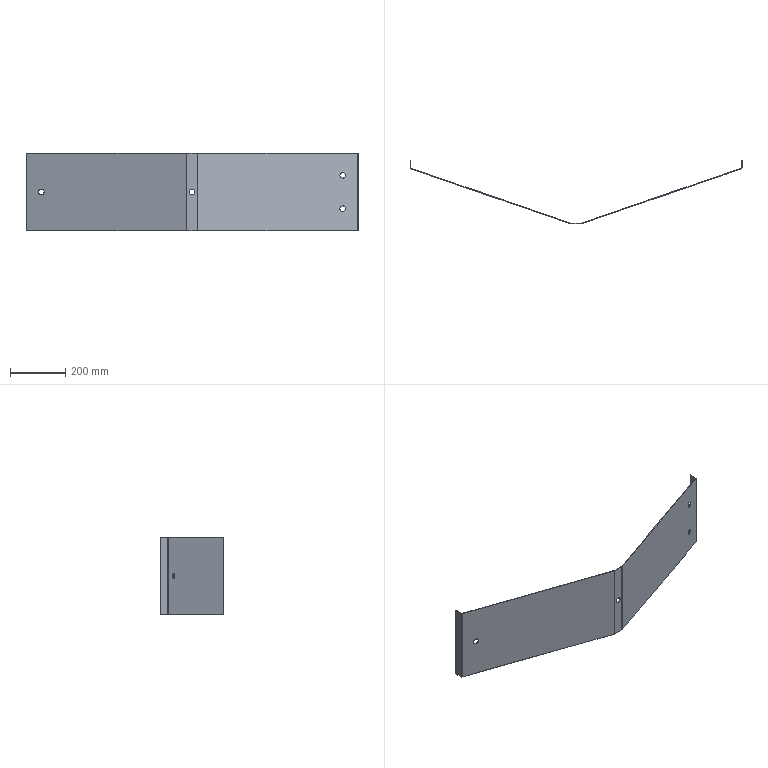Part | SolidWorks | features ICE 4, FlatPattern 1, SMBaseFlange 1, SheetMetal 1 | 1 solid | 46 faces | box 1200 x 230 x 280 mm | volume 738116 mm3 | plane 30 | cylinder 16 | commonest cylinder face diameters 20 x8 2 x4 6 x4
STEP:
#1=CARTESIAN_POINT('',(55.332,-16.965,130.));
#2=VERTEX_POINT('',#1);
#3=CARTESIAN_POINT('',(55.332,-16.965,150.));
#4=VERTEX_POINT('',#3);
#5=CARTESIAN_POINT('',(55.332,-16.965,130.));
#6=CARTESIAN_POINT('',(35.332,-10.068,130.));
#7=CARTESIAN_POINT('',(35.332,-10.068,150.));
#8=CARTESIAN_POINT('',(55.332,-16.965,150.));
#9=(BOUNDED_CURVE()B_SPLINE_CURVE(3,(#5,#6,#7,#8),.UNSPECIFIED.,.F.,.T.)B_SPLINE_CURVE_WITH_KNOTS((4,4),(1.571,4.712),.UNSPECIFIED.)CURVE()GEOMETRIC_REPRESENTATION_ITEM()RATIONAL_B_SPLINE_CURVE((1.,0.3333,0.3333,1.))REPRESENTATION_ITEM(''));
#10=EDGE_CURVE('',#2,#4,#9,.T.);
#11=ORIENTED_EDGE('',*,*,#10,.T.);
#12=CARTESIAN_POINT('',(55.332,-19.08,150.));
#13=VERTEX_POINT('',#12);
#14=CARTESIAN_POINT('',(55.332,30.,150.));
#15=DIRECTION('',(0.,-1.,0.));
#16=VECTOR('',#15,1000.);
#17=LINE('',#14,#16);
#18=EDGE_CURVE('',#4,#13,#17,.T.);
#19=ORIENTED_EDGE('',*,*,#18,.T.);
#20=CARTESIAN_POINT('',(55.332,-19.08,130.));
#21=VERTEX_POINT('',#20);
#22=CARTESIAN_POINT('',(55.332,-19.08,130.));
#23=CARTESIAN_POINT('',(35.332,-12.184,130.));
#24=CARTESIAN_POINT('',(35.332,-12.184,150.));
#25=CARTESIAN_POINT('',(55.332,-19.08,150.));
#26=(BOUNDED_CURVE()B_SPLINE_CURVE(3,(#22,#23,#24,#25),.UNSPECIFIED.,.F.,.F.)B_SPLINE_CURVE_WITH_KNOTS((4,4),(1.571,4.712),.UNSPECIFIED.)CURVE()GEOMETRIC_REPRESENTATION_ITEM()RATIONAL_B_SPLINE_CURVE((1.,0.3333,0.3333,1.))REPRESENTATION_ITEM(''));
#27=EDGE_CURVE('',#21,#13,#26,.T.);
#28=ORIENTED_EDGE('',*,*,#27,.F.);
#29=CARTESIAN_POINT('',(55.332,30.,130.));
#30=DIRECTION('',(0.,-1.,0.));
#31=VECTOR('',#30,1000.);
#32=LINE('',#29,#31);
#33=EDGE_CURVE('',#2,#21,#32,.T.);
#34=ORIENTED_EDGE('',*,*,#33,.F.);
#35=EDGE_LOOP('',(#11,#19,#28,#34));
#36=FACE_OUTER_BOUND('',#35,.T.);
#37=CARTESIAN_POINT('',(55.332,30.,140.));
#38=DIRECTION('',(0.,-1.,0.));
#39=DIRECTION('',(0.,0.,-1.));
#40=AXIS2_PLACEMENT_3D('',#37,#38,#39);
#41=CYLINDRICAL_SURFACE('',#40,10.);
#42=ADVANCED_FACE('',(#36),#41,.F.);
#43=CARTESIAN_POINT('',(1144.668,-16.965,190.));
#44=VERTEX_POINT('',#43);
#45=CARTESIAN_POINT('',(1144.668,-16.965,210.));
#46=VERTEX_POINT('',#45);
#47=CARTESIAN_POINT('',(1144.668,-16.965,190.));
#48=CARTESIAN_POINT('',(1124.668,-23.861,190.));
#49=CARTESIAN_POINT('',(1124.668,-23.861,210.));
#50=CARTESIAN_POINT('',(1144.668,-16.965,210.));
#51=(BOUNDED_CURVE()B_SPLINE_CURVE(3,(#47,#48,#49,#50),.UNSPECIFIED.,.F.,.T.)B_SPLINE_CURVE_WITH_KNOTS((4,4),(4.712,7.854),.UNSPECIFIED.)CURVE()GEOMETRIC_REPRESENTATION_ITEM()RATIONAL_B_SPLINE_CURVE((1.,0.3333,0.3333,1.))REPRESENTATION_ITEM(''));
#52=EDGE_CURVE('',#44,#46,#51,.T.);
#53=ORIENTED_EDGE('',*,*,#52,.T.);
#54=CARTESIAN_POINT('',(1144.668,-19.08,210.));
#55=VERTEX_POINT('',#54);
#56=CARTESIAN_POINT('',(1144.668,30.,210.));
#57=DIRECTION('',(0.,-1.,0.));
#58=VECTOR('',#57,1000.);
#59=LINE('',#56,#58);
#60=EDGE_CURVE('',#46,#55,#59,.T.);
#61=ORIENTED_EDGE('',*,*,#60,.T.);
#62=CARTESIAN_POINT('',(1144.668,-19.08,190.));
#63=VERTEX_POINT('',#62);
#64=CARTESIAN_POINT('',(1144.668,-19.08,190.));
#65=CARTESIAN_POINT('',(1124.668,-25.977,190.));
#66=CARTESIAN_POINT('',(1124.668,-25.977,210.));
#67=CARTESIAN_POINT('',(1144.668,-19.08,210.));
#68=(BOUNDED_CURVE()B_SPLINE_CURVE(3,(#64,#65,#66,#67),.UNSPECIFIED.,.F.,.F.)B_SPLINE_CURVE_WITH_KNOTS((4,4),(4.712,7.854),.UNSPECIFIED.)CURVE()GEOMETRIC_REPRESENTATION_ITEM()RATIONAL_B_SPLINE_CURVE((1.,0.3333,0.3333,1.))REPRESENTATION_ITEM(''));
#69=EDGE_CURVE('',#63,#55,#68,.T.);
#70=ORIENTED_EDGE('',*,*,#69,.F.);
#71=CARTESIAN_POINT('',(1144.668,30.,190.));
#72=DIRECTION('',(0.,-1.,0.));
#73=VECTOR('',#72,1000.);
#74=LINE('',#71,#73);
#75=EDGE_CURVE('',#44,#63,#74,.T.);
#76=ORIENTED_EDGE('',*,*,#75,.F.);
#77=EDGE_LOOP('',(#53,#61,#70,#76));
#78=FACE_OUTER_BOUND('',#77,.T.);
#79=CARTESIAN_POINT('',(1144.668,30.,200.));
#80=DIRECTION('',(0.,-1.,0.));
#81=DIRECTION('',(0.,0.,-1.));
#82=AXIS2_PLACEMENT_3D('',#79,#80,#81);
#83=CYLINDRICAL_SURFACE('',#82,10.);
#84=ADVANCED_FACE('',(#78),#83,.F.);
#85=CARTESIAN_POINT('',(1144.668,-16.965,70.));
#86=VERTEX_POINT('',#85);
#87=CARTESIAN_POINT('',(1144.668,-16.965,90.));
#88=VERTEX_POINT('',#87);
#89=CARTESIAN_POINT('',(1144.668,-16.965,70.));
#90=CARTESIAN_POINT('',(1124.668,-23.861,70.));
#91=CARTESIAN_POINT('',(1124.668,-23.861,90.));
#92=CARTESIAN_POINT('',(1144.668,-16.965,90.));
#93=(BOUNDED_CURVE()B_SPLINE_CURVE(3,(#89,#90,#91,#92),.UNSPECIFIED.,.F.,.T.)B_SPLINE_CURVE_WITH_KNOTS((4,4),(4.712,7.854),.UNSPECIFIED.)CURVE()GEOMETRIC_REPRESENTATION_ITEM()RATIONAL_B_SPLINE_CURVE((1.,0.3333,0.3333,1.))REPRESENTATION_ITEM(''));
#94=EDGE_CURVE('',#86,#88,#93,.T.);
#95=ORIENTED_EDGE('',*,*,#94,.T.);
#96=CARTESIAN_POINT('',(1144.668,-19.08,90.));
#97=VERTEX_POINT('',#96);
#98=CARTESIAN_POINT('',(1144.668,30.,90.));
#99=DIRECTION('',(0.,-1.,0.));
#100=VECTOR('',#99,1000.);
#101=LINE('',#98,#100);
#102=EDGE_CURVE('',#88,#97,#101,.T.);
#103=ORIENTED_EDGE('',*,*,#102,.T.);
#104=CARTESIAN_POINT('',(1144.668,-19.08,70.));
#105=VERTEX_POINT('',#104);
#106=CARTESIAN_POINT('',(1144.668,-19.08,70.));
#107=CARTESIAN_POINT('',(1124.668,-25.977,70.));
#108=CARTESIAN_POINT('',(1124.668,-25.977,90.));
#109=CARTESIAN_POINT('',(1144.668,-19.08,90.));
#110=(BOUNDED_CURVE()B_SPLINE_CURVE(3,(#106,#107,#108,#109),.UNSPECIFIED.,.F.,.F.)B_SPLINE_CURVE_WITH_KNOTS((4,4),(4.712,7.854),.UNSPECIFIED.)CURVE()GEOMETRIC_REPRESENTATION_ITEM()RATIONAL_B_SPLINE_CURVE((1.,0.3333,0.3333,1.))REPRESENTATION_ITEM(''));
#111=EDGE_CURVE('',#105,#97,#110,.T.);
#112=ORIENTED_EDGE('',*,*,#111,.F.);
#113=CARTESIAN_POINT('',(1144.668,30.,70.));
#114=DIRECTION('',(0.,-1.,0.));
#115=VECTOR('',#114,1000.);
#116=LINE('',#113,#115);
#117=EDGE_CURVE('',#86,#105,#116,.T.);
#118=ORIENTED_EDGE('',*,*,#117,.F.);
#119=EDGE_LOOP('',(#95,#103,#112,#118));
#120=FACE_OUTER_BOUND('',#119,.T.);
#121=CARTESIAN_POINT('',(1144.668,30.,80.));
#122=DIRECTION('',(0.,-1.,0.));
#123=DIRECTION('',(0.,0.,-1.));
#124=AXIS2_PLACEMENT_3D('',#121,#122,#123);
#125=CYLINDRICAL_SURFACE('',#124,10.);
#126=ADVANCED_FACE('',(#120),#125,.F.);
#127=CARTESIAN_POINT('',(600.,-200.,130.));
#128=VERTEX_POINT('',#127);
#129=CARTESIAN_POINT('',(600.,-200.,150.));
#130=VERTEX_POINT('',#129);
#131=CARTESIAN_POINT('',(600.,-200.,140.));
#132=DIRECTION('',(0.,1.,0.));
#133=DIRECTION('',(0.,0.,1.));
#134=AXIS2_PLACEMENT_3D('',#131,#132,#133);
#135=CIRCLE('',#134,10.);
#136=EDGE_CURVE('',#128,#130,#135,.T.);
#137=ORIENTED_EDGE('',*,*,#136,.F.);
#138=CARTESIAN_POINT('',(600.,-198.,130.));
#139=VERTEX_POINT('',#138);
#140=CARTESIAN_POINT('',(600.,-208.,130.));
#141=DIRECTION('',(0.,1.,0.));
#142=VECTOR('',#141,1000.);
#143=LINE('',#140,#142);
#144=EDGE_CURVE('',#128,#139,#143,.T.);
#145=ORIENTED_EDGE('',*,*,#144,.T.);
#146=CARTESIAN_POINT('',(600.,-198.,150.));
#147=VERTEX_POINT('',#146);
#148=CARTESIAN_POINT('',(600.,-198.,140.));
#149=DIRECTION('',(0.,1.,0.));
#150=DIRECTION('',(0.,0.,1.));
#151=AXIS2_PLACEMENT_3D('',#148,#149,#150);
#152=CIRCLE('',#151,10.);
#153=EDGE_CURVE('',#139,#147,#152,.T.);
#154=ORIENTED_EDGE('',*,*,#153,.T.);
#155=CARTESIAN_POINT('',(600.,-208.,150.));
#156=DIRECTION('',(0.,1.,0.));
#157=VECTOR('',#156,1000.);
#158=LINE('',#155,#157);
#159=EDGE_CURVE('',#130,#147,#158,.T.);
#160=ORIENTED_EDGE('',*,*,#159,.F.);
#161=EDGE_LOOP('',(#137,#145,#154,#160));
#162=FACE_OUTER_BOUND('',#161,.T.);
#163=CARTESIAN_POINT('',(600.,-208.,140.));
#164=DIRECTION('',(0.,1.,0.));
#165=DIRECTION('',(0.,0.,1.));
#166=AXIS2_PLACEMENT_3D('',#163,#164,#165);
#167=CYLINDRICAL_SURFACE('',#166,10.);
#168=ADVANCED_FACE('',(#162),#167,.F.);
#169=CARTESIAN_POINT('',(0.,2.139,280.));
#170=VERTEX_POINT('',#169);
#171=CARTESIAN_POINT('',(2.,2.139,280.));
#172=VERTEX_POINT('',#171);
#173=CARTESIAN_POINT('',(0.,2.139,280.));
#174=DIRECTION('',(1.,0.,0.));
#175=VECTOR('',#174,1000.);
#176=LINE('',#173,#175);
#177=EDGE_CURVE('',#170,#172,#176,.T.);
#178=ORIENTED_EDGE('',*,*,#177,.F.);
#179=CARTESIAN_POINT('',(2.022,-0.6973,280.));
#180=VERTEX_POINT('',#179);
#181=CARTESIAN_POINT('',(3.,2.139,280.));
#182=DIRECTION('',(0.,0.,1.));
#183=DIRECTION('',(-1.,0.,0.));
#184=AXIS2_PLACEMENT_3D('',#181,#182,#183);
#185=CIRCLE('',#184,3.);
#186=EDGE_CURVE('',#170,#180,#185,.T.);
#187=ORIENTED_EDGE('',*,*,#186,.T.);
#188=CARTESIAN_POINT('',(2.674,1.193,280.));
#189=VERTEX_POINT('',#188);
#190=CARTESIAN_POINT('',(2.674,1.193,280.));
#191=DIRECTION('',(-0.326,-0.9454,0.));
#192=VECTOR('',#191,1000.);
#193=LINE('',#190,#192);
#194=EDGE_CURVE('',#189,#180,#193,.T.);
#195=ORIENTED_EDGE('',*,*,#194,.F.);
#196=CARTESIAN_POINT('',(3.,2.139,280.));
#197=DIRECTION('',(0.,0.,1.));
#198=DIRECTION('',(1.,0.,0.));
#199=AXIS2_PLACEMENT_3D('',#196,#197,#198);
#200=CIRCLE('',#199,1.);
#201=EDGE_CURVE('',#172,#189,#200,.T.);
#202=ORIENTED_EDGE('',*,*,#201,.F.);
#203=EDGE_LOOP('',(#178,#187,#195,#202));
#204=FACE_OUTER_BOUND('',#203,.T.);
#205=CARTESIAN_POINT('',(0.,2.139,280.));
#206=DIRECTION('',(0.,0.,1.));
#207=DIRECTION('',(1.,0.,0.));
#208=AXIS2_PLACEMENT_3D('',#205,#206,#207);
#209=PLANE('',#208);
#210=ADVANCED_FACE('',(#204),#209,.T.);
#211=CARTESIAN_POINT('',(0.,30.,280.));
#212=VERTEX_POINT('',#211);
#213=CARTESIAN_POINT('',(0.,0.,280.));
#214=DIRECTION('',(0.,-1.,0.));
#215=VECTOR('',#214,1000.);
#216=LINE('',#213,#215);
#217=EDGE_CURVE('',#212,#170,#216,.T.);
#218=ORIENTED_EDGE('',*,*,#217,.T.);
#219=ORIENTED_EDGE('',*,*,#177,.T.);
#220=CARTESIAN_POINT('',(2.,30.,280.));
#221=VERTEX_POINT('',#220);
#222=CARTESIAN_POINT('',(2.,0.,280.));
#223=DIRECTION('',(0.,-1.,0.));
#224=VECTOR('',#223,1000.);
#225=LINE('',#222,#224);
#226=EDGE_CURVE('',#221,#172,#225,.T.);
#227=ORIENTED_EDGE('',*,*,#226,.F.);
#228=CARTESIAN_POINT('',(0.,30.,280.));
#229=DIRECTION('',(1.,0.,0.));
#230=VECTOR('',#229,1000.);
#231=LINE('',#228,#230);
#232=EDGE_CURVE('',#212,#221,#231,.T.);
#233=ORIENTED_EDGE('',*,*,#232,.F.);
#234=EDGE_LOOP('',(#218,#219,#227,#233));
#235=FACE_OUTER_BOUND('',#234,.T.);
#236=CARTESIAN_POINT('',(2.674,1.193,280.));
#237=DIRECTION('',(0.,0.,1.));
#238=DIRECTION('',(1.,0.,0.));
#239=AXIS2_PLACEMENT_3D('',#236,#237,#238);
#240=PLANE('',#239);
#241=ADVANCED_FACE('',(#235),#240,.T.);
#242=CARTESIAN_POINT('',(2.022,-0.6973,0.));
#243=VERTEX_POINT('',#242);
#244=CARTESIAN_POINT('',(2.674,1.193,0.));
#245=VERTEX_POINT('',#244);
#246=CARTESIAN_POINT('',(2.022,-0.6973,0.));
#247=DIRECTION('',(0.326,0.9454,0.));
#248=VECTOR('',#247,1000.);
#249=LINE('',#246,#248);
#250=EDGE_CURVE('',#243,#245,#249,.T.);
#251=ORIENTED_EDGE('',*,*,#250,.F.);
#252=CARTESIAN_POINT('',(0.,2.139,0.));
#253=VERTEX_POINT('',#252);
#254=CARTESIAN_POINT('',(3.,2.139,0.));
#255=DIRECTION('',(0.,0.,1.));
#256=DIRECTION('',(-1.,0.,0.));
#257=AXIS2_PLACEMENT_3D('',#254,#255,#256);
#258=CIRCLE('',#257,3.);
#259=EDGE_CURVE('',#253,#243,#258,.T.);
#260=ORIENTED_EDGE('',*,*,#259,.F.);
#261=CARTESIAN_POINT('',(2.,2.139,0.));
#262=VERTEX_POINT('',#261);
#263=CARTESIAN_POINT('',(2.,2.139,0.));
#264=DIRECTION('',(-1.,0.,0.));
#265=VECTOR('',#264,1000.);
#266=LINE('',#263,#265);
#267=EDGE_CURVE('',#262,#253,#266,.T.);
#268=ORIENTED_EDGE('',*,*,#267,.F.);
#269=CARTESIAN_POINT('',(3.,2.139,0.));
#270=DIRECTION('',(0.,0.,1.));
#271=DIRECTION('',(1.,0.,0.));
#272=AXIS2_PLACEMENT_3D('',#269,#270,#271);
#273=CIRCLE('',#272,1.);
#274=EDGE_CURVE('',#262,#245,#273,.T.);
#275=ORIENTED_EDGE('',*,*,#274,.T.);
#276=EDGE_LOOP('',(#251,#260,#268,#275));
#277=FACE_OUTER_BOUND('',#276,.T.);
#278=CARTESIAN_POINT('',(2.022,-0.6973,0.));
#279=DIRECTION('',(0.,0.,-1.));
#280=DIRECTION('',(-1.,0.,0.));
#281=AXIS2_PLACEMENT_3D('',#278,#279,#280);
#282=PLANE('',#281);
#283=ADVANCED_FACE('',(#277),#282,.T.);
#284=CARTESIAN_POINT('',(579.525,-199.836,0.));
#285=VERTEX_POINT('',#284);
#286=CARTESIAN_POINT('',(0.,0.,0.));
#287=DIRECTION('',(0.9454,-0.326,0.));
#288=VECTOR('',#287,1000.);
#289=LINE('',#286,#288);
#290=EDGE_CURVE('',#243,#285,#289,.T.);
#291=ORIENTED_EDGE('',*,*,#290,.F.);
#292=ORIENTED_EDGE('',*,*,#250,.T.);
#293=CARTESIAN_POINT('',(580.177,-197.945,0.));
#294=VERTEX_POINT('',#293);
#295=CARTESIAN_POINT('',(0.652,1.891,0.));
#296=DIRECTION('',(0.9454,-0.326,0.));
#297=VECTOR('',#296,1000.);
#298=LINE('',#295,#297);
#299=EDGE_CURVE('',#245,#294,#298,.T.);
#300=ORIENTED_EDGE('',*,*,#299,.T.);
#301=CARTESIAN_POINT('',(580.177,-197.945,0.));
#302=DIRECTION('',(-0.326,-0.9454,0.));
#303=VECTOR('',#302,1000.);
#304=LINE('',#301,#303);
#305=EDGE_CURVE('',#294,#285,#304,.T.);
#306=ORIENTED_EDGE('',*,*,#305,.T.);
#307=EDGE_LOOP('',(#291,#292,#300,#306));
#308=FACE_OUTER_BOUND('',#307,.T.);
#309=CARTESIAN_POINT('',(2.,2.139,0.));
#310=DIRECTION('',(0.,0.,-1.));
#311=DIRECTION('',(-1.,0.,0.));
#312=AXIS2_PLACEMENT_3D('',#309,#310,#311);
#313=PLANE('',#312);
#314=ADVANCED_FACE('',(#308),#313,.T.);
#315=CARTESIAN_POINT('',(579.525,-199.836,280.));
#316=VERTEX_POINT('',#315);
#317=CARTESIAN_POINT('',(580.177,-197.945,280.));
#318=VERTEX_POINT('',#317);
#319=CARTESIAN_POINT('',(579.525,-199.836,280.));
#320=DIRECTION('',(0.326,0.9454,0.));
#321=VECTOR('',#320,1000.);
#322=LINE('',#319,#321);
#323=EDGE_CURVE('',#316,#318,#322,.T.);
#324=ORIENTED_EDGE('',*,*,#323,.F.);
#325=CARTESIAN_POINT('',(580.503,-200.,280.));
#326=VERTEX_POINT('',#325);
#327=CARTESIAN_POINT('',(580.503,-197.,280.));
#328=DIRECTION('',(0.,0.,1.));
#329=DIRECTION('',(-1.,0.,0.));
#330=AXIS2_PLACEMENT_3D('',#327,#328,#329);
#331=CIRCLE('',#330,3.);
#332=EDGE_CURVE('',#316,#326,#331,.T.);
#333=ORIENTED_EDGE('',*,*,#332,.T.);
#334=CARTESIAN_POINT('',(580.503,-198.,280.));
#335=VERTEX_POINT('',#334);
#336=CARTESIAN_POINT('',(580.503,-198.,280.));
#337=DIRECTION('',(0.,-1.,0.));
#338=VECTOR('',#337,1000.);
#339=LINE('',#336,#338);
#340=EDGE_CURVE('',#335,#326,#339,.T.);
#341=ORIENTED_EDGE('',*,*,#340,.F.);
#342=CARTESIAN_POINT('',(580.503,-197.,280.));
#343=DIRECTION('',(0.,0.,1.));
#344=DIRECTION('',(1.,0.,0.));
#345=AXIS2_PLACEMENT_3D('',#342,#343,#344);
#346=CIRCLE('',#345,1.);
#347=EDGE_CURVE('',#318,#335,#346,.T.);
#348=ORIENTED_EDGE('',*,*,#347,.F.);
#349=EDGE_LOOP('',(#324,#333,#341,#348));
#350=FACE_OUTER_BOUND('',#349,.T.);
#351=CARTESIAN_POINT('',(579.525,-199.836,280.));
#352=DIRECTION('',(0.,0.,1.));
#353=DIRECTION('',(1.,0.,0.));
#354=AXIS2_PLACEMENT_3D('',#351,#352,#353);
#355=PLANE('',#354);
#356=ADVANCED_FACE('',(#350),#355,.T.);
#357=CARTESIAN_POINT('',(0.,0.,280.));
#358=DIRECTION('',(0.9454,-0.326,0.));
#359=VECTOR('',#358,1000.);
#360=LINE('',#357,#359);
#361=EDGE_CURVE('',#180,#316,#360,.T.);
#362=ORIENTED_EDGE('',*,*,#361,.T.);
#363=ORIENTED_EDGE('',*,*,#323,.T.);
#364=CARTESIAN_POINT('',(0.652,1.891,280.));
#365=DIRECTION('',(0.9454,-0.326,0.));
#366=VECTOR('',#365,1000.);
#367=LINE('',#364,#366);
#368=EDGE_CURVE('',#189,#318,#367,.T.);
#369=ORIENTED_EDGE('',*,*,#368,.F.);
#370=ORIENTED_EDGE('',*,*,#194,.T.);
#371=EDGE_LOOP('',(#362,#363,#369,#370));
#372=FACE_OUTER_BOUND('',#371,.T.);
#373=CARTESIAN_POINT('',(580.503,-198.,280.));
#374=DIRECTION('',(0.,0.,1.));
#375=DIRECTION('',(1.,0.,0.));
#376=AXIS2_PLACEMENT_3D('',#373,#374,#375);
#377=PLANE('',#376);
#378=ADVANCED_FACE('',(#372),#377,.T.);
#379=CARTESIAN_POINT('',(580.503,-200.,0.));
#380=VERTEX_POINT('',#379);
#381=CARTESIAN_POINT('',(580.503,-198.,0.));
#382=VERTEX_POINT('',#381);
#383=CARTESIAN_POINT('',(580.503,-200.,0.));
#384=DIRECTION('',(0.,1.,0.));
#385=VECTOR('',#384,1000.);
#386=LINE('',#383,#385);
#387=EDGE_CURVE('',#380,#382,#386,.T.);
#388=ORIENTED_EDGE('',*,*,#387,.F.);
#389=CARTESIAN_POINT('',(580.503,-197.,0.));
#390=DIRECTION('',(0.,0.,1.));
#391=DIRECTION('',(-1.,0.,0.));
#392=AXIS2_PLACEMENT_3D('',#389,#390,#391);
#393=CIRCLE('',#392,3.);
#394=EDGE_CURVE('',#285,#380,#393,.T.);
#395=ORIENTED_EDGE('',*,*,#394,.F.);
#396=ORIENTED_EDGE('',*,*,#305,.F.);
#397=CARTESIAN_POINT('',(580.503,-197.,0.));
#398=DIRECTION('',(0.,0.,1.));
#399=DIRECTION('',(1.,0.,0.));
#400=AXIS2_PLACEMENT_3D('',#397,#398,#399);
#401=CIRCLE('',#400,1.);
#402=EDGE_CURVE('',#294,#382,#401,.T.);
#403=ORIENTED_EDGE('',*,*,#402,.T.);
#404=EDGE_LOOP('',(#388,#395,#396,#403));
#405=FACE_OUTER_BOUND('',#404,.T.);
#406=CARTESIAN_POINT('',(580.503,-200.,0.));
#407=DIRECTION('',(0.,0.,-1.));
#408=DIRECTION('',(-1.,0.,0.));
#409=AXIS2_PLACEMENT_3D('',#406,#407,#408);
#410=PLANE('',#409);
#411=ADVANCED_FACE('',(#405),#410,.T.);
#412=CARTESIAN_POINT('',(619.497,-200.,0.));
#413=VERTEX_POINT('',#412);
#414=CARTESIAN_POINT('',(580.,-200.,0.));
#415=DIRECTION('',(1.,0.,0.));
#416=VECTOR('',#415,1000.);
#417=LINE('',#414,#416);
#418=EDGE_CURVE('',#380,#413,#417,.T.);
#419=ORIENTED_EDGE('',*,*,#418,.F.);
#420=ORIENTED_EDGE('',*,*,#387,.T.);
#421=CARTESIAN_POINT('',(619.497,-198.,0.));
#422=VERTEX_POINT('',#421);
#423=CARTESIAN_POINT('',(580.,-198.,0.));
#424=DIRECTION('',(1.,0.,0.));
#425=VECTOR('',#424,1000.);
#426=LINE('',#423,#425);
#427=EDGE_CURVE('',#382,#422,#426,.T.);
#428=ORIENTED_EDGE('',*,*,#427,.T.);
#429=CARTESIAN_POINT('',(619.497,-198.,0.));
#430=DIRECTION('',(0.,-1.,0.));
#431=VECTOR('',#430,1000.);
#432=LINE('',#429,#431);
#433=EDGE_CURVE('',#422,#413,#432,.T.);
#434=ORIENTED_EDGE('',*,*,#433,.T.);
#435=EDGE_LOOP('',(#419,#420,#428,#434));
#436=FACE_OUTER_BOUND('',#435,.T.);
#437=CARTESIAN_POINT('',(580.177,-197.945,0.));
#438=DIRECTION('',(0.,0.,-1.));
#439=DIRECTION('',(-1.,0.,0.));
#440=AXIS2_PLACEMENT_3D('',#437,#438,#439);
#441=PLANE('',#440);
#442=ADVANCED_FACE('',(#436),#441,.T.);
#443=CARTESIAN_POINT('',(619.497,-200.,280.));
#444=VERTEX_POINT('',#443);
#445=CARTESIAN_POINT('',(619.497,-198.,280.));
#446=VERTEX_POINT('',#445);
#447=CARTESIAN_POINT('',(619.497,-200.,280.));
#448=DIRECTION('',(0.,1.,0.));
#449=VECTOR('',#448,1000.);
#450=LINE('',#447,#449);
#451=EDGE_CURVE('',#444,#446,#450,.T.);
#452=ORIENTED_EDGE('',*,*,#451,.F.);
#453=CARTESIAN_POINT('',(620.475,-199.836,280.));
#454=VERTEX_POINT('',#453);
#455=CARTESIAN_POINT('',(619.497,-197.,280.));
#456=DIRECTION('',(0.,0.,1.));
#457=DIRECTION('',(-1.,0.,0.));
#458=AXIS2_PLACEMENT_3D('',#455,#456,#457);
#459=CIRCLE('',#458,3.);
#460=EDGE_CURVE('',#444,#454,#459,.T.);
#461=ORIENTED_EDGE('',*,*,#460,.T.);
#462=CARTESIAN_POINT('',(619.823,-197.945,280.));
#463=VERTEX_POINT('',#462);
#464=CARTESIAN_POINT('',(619.823,-197.945,280.));
#465=DIRECTION('',(0.326,-0.9454,0.));
#466=VECTOR('',#465,1000.);
#467=LINE('',#464,#466);
#468=EDGE_CURVE('',#463,#454,#467,.T.);
#469=ORIENTED_EDGE('',*,*,#468,.F.);
#470=CARTESIAN_POINT('',(619.497,-197.,280.));
#471=DIRECTION('',(0.,0.,1.));
#472=DIRECTION('',(1.,0.,0.));
#473=AXIS2_PLACEMENT_3D('',#470,#471,#472);
#474=CIRCLE('',#473,1.);
#475=EDGE_CURVE('',#446,#463,#474,.T.);
#476=ORIENTED_EDGE('',*,*,#475,.F.);
#477=EDGE_LOOP('',(#452,#461,#469,#476));
#478=FACE_OUTER_BOUND('',#477,.T.);
#479=CARTESIAN_POINT('',(619.497,-200.,280.));
#480=DIRECTION('',(0.,0.,1.));
#481=DIRECTION('',(1.,0.,0.));
#482=AXIS2_PLACEMENT_3D('',#479,#480,#481);
#483=PLANE('',#482);
#484=ADVANCED_FACE('',(#478),#483,.T.);
#485=CARTESIAN_POINT('',(580.,-200.,280.));
#486=DIRECTION('',(1.,0.,0.));
#487=VECTOR('',#486,1000.);
#488=LINE('',#485,#487);
#489=EDGE_CURVE('',#326,#444,#488,.T.);
#490=ORIENTED_EDGE('',*,*,#489,.T.);
#491=ORIENTED_EDGE('',*,*,#451,.T.);
#492=CARTESIAN_POINT('',(580.,-198.,280.));
#493=DIRECTION('',(1.,0.,0.));
#494=VECTOR('',#493,1000.);
#495=LINE('',#492,#494);
#496=EDGE_CURVE('',#335,#446,#495,.T.);
#497=ORIENTED_EDGE('',*,*,#496,.F.);
#498=ORIENTED_EDGE('',*,*,#340,.T.);
#499=EDGE_LOOP('',(#490,#491,#497,#498));
#500=FACE_OUTER_BOUND('',#499,.T.);
#501=CARTESIAN_POINT('',(619.823,-197.945,280.));
#502=DIRECTION('',(0.,0.,1.));
#503=DIRECTION('',(1.,0.,0.));
#504=AXIS2_PLACEMENT_3D('',#501,#502,#503);
#505=PLANE('',#504);
#506=ADVANCED_FACE('',(#500),#505,.T.);
#507=CARTESIAN_POINT('',(620.475,-199.836,0.));
#508=VERTEX_POINT('',#507);
#509=CARTESIAN_POINT('',(619.823,-197.945,0.));
#510=VERTEX_POINT('',#509);
#511=CARTESIAN_POINT('',(620.475,-199.836,0.));
#512=DIRECTION('',(-0.326,0.9454,0.));
#513=VECTOR('',#512,1000.);
#514=LINE('',#511,#513);
#515=EDGE_CURVE('',#508,#510,#514,.T.);
#516=ORIENTED_EDGE('',*,*,#515,.F.);
#517=CARTESIAN_POINT('',(619.497,-197.,0.));
#518=DIRECTION('',(0.,0.,1.));
#519=DIRECTION('',(-1.,0.,0.));
#520=AXIS2_PLACEMENT_3D('',#517,#518,#519);
#521=CIRCLE('',#520,3.);
#522=EDGE_CURVE('',#413,#508,#521,.T.);
#523=ORIENTED_EDGE('',*,*,#522,.F.);
#524=ORIENTED_EDGE('',*,*,#433,.F.);
#525=CARTESIAN_POINT('',(619.497,-197.,0.));
#526=DIRECTION('',(0.,0.,1.));
#527=DIRECTION('',(1.,0.,0.));
#528=AXIS2_PLACEMENT_3D('',#525,#526,#527);
#529=CIRCLE('',#528,1.);
#530=EDGE_CURVE('',#422,#510,#529,.T.);
#531=ORIENTED_EDGE('',*,*,#530,.T.);
#532=EDGE_LOOP('',(#516,#523,#524,#531));
#533=FACE_OUTER_BOUND('',#532,.T.);
#534=CARTESIAN_POINT('',(620.475,-199.836,0.));
#535=DIRECTION('',(0.,0.,-1.));
#536=DIRECTION('',(-1.,0.,0.));
#537=AXIS2_PLACEMENT_3D('',#534,#535,#536);
#538=PLANE('',#537);
#539=ADVANCED_FACE('',(#533),#538,.T.);
#540=CARTESIAN_POINT('',(1197.978,-0.6973,0.));
#541=VERTEX_POINT('',#540);
#542=CARTESIAN_POINT('',(620.,-200.,0.));
#543=DIRECTION('',(0.9454,0.326,0.));
#544=VECTOR('',#543,1000.);
#545=LINE('',#542,#544);
#546=EDGE_CURVE('',#508,#541,#545,.T.);
#547=ORIENTED_EDGE('',*,*,#546,.F.);
#548=ORIENTED_EDGE('',*,*,#515,.T.);
#549=CARTESIAN_POINT('',(1197.326,1.193,0.));
#550=VERTEX_POINT('',#549);
#551=CARTESIAN_POINT('',(619.348,-198.109,0.));
#552=DIRECTION('',(0.9454,0.326,0.));
#553=VECTOR('',#552,1000.);
#554=LINE('',#551,#553);
#555=EDGE_CURVE('',#510,#550,#554,.T.);
#556=ORIENTED_EDGE('',*,*,#555,.T.);
#557=CARTESIAN_POINT('',(1197.326,1.193,0.));
#558=DIRECTION('',(0.326,-0.9454,0.));
#559=VECTOR('',#558,1000.);
#560=LINE('',#557,#559);
#561=EDGE_CURVE('',#550,#541,#560,.T.);
#562=ORIENTED_EDGE('',*,*,#561,.T.);
#563=EDGE_LOOP('',(#547,#548,#556,#562));
#564=FACE_OUTER_BOUND('',#563,.T.);
#565=CARTESIAN_POINT('',(619.497,-198.,0.));
#566=DIRECTION('',(0.,0.,-1.));
#567=DIRECTION('',(-1.,0.,0.));
#568=AXIS2_PLACEMENT_3D('',#565,#566,#567);
#569=PLANE('',#568);
#570=ADVANCED_FACE('',(#564),#569,.T.);
#571=CARTESIAN_POINT('',(1197.978,-0.6973,280.));
#572=VERTEX_POINT('',#571);
#573=CARTESIAN_POINT('',(1197.326,1.193,280.));
#574=VERTEX_POINT('',#573);
#575=CARTESIAN_POINT('',(1197.978,-0.6973,280.));
#576=DIRECTION('',(-0.326,0.9454,0.));
#577=VECTOR('',#576,1000.);
#578=LINE('',#575,#577);
#579=EDGE_CURVE('',#572,#574,#578,.T.);
#580=ORIENTED_EDGE('',*,*,#579,.F.);
#581=CARTESIAN_POINT('',(1200.,2.139,280.));
#582=VERTEX_POINT('',#581);
#583=CARTESIAN_POINT('',(1197.,2.139,280.));
#584=DIRECTION('',(0.,0.,1.));
#585=DIRECTION('',(-1.,0.,0.));
#586=AXIS2_PLACEMENT_3D('',#583,#584,#585);
#587=CIRCLE('',#586,3.);
#588=EDGE_CURVE('',#572,#582,#587,.T.);
#589=ORIENTED_EDGE('',*,*,#588,.T.);
#590=CARTESIAN_POINT('',(1198.,2.139,280.));
#591=VERTEX_POINT('',#590);
#592=CARTESIAN_POINT('',(1198.,2.139,280.));
#593=DIRECTION('',(1.,0.,0.));
#594=VECTOR('',#593,1000.);
#595=LINE('',#592,#594);
#596=EDGE_CURVE('',#591,#582,#595,.T.);
#597=ORIENTED_EDGE('',*,*,#596,.F.);
#598=CARTESIAN_POINT('',(1197.,2.139,280.));
#599=DIRECTION('',(0.,0.,1.));
#600=DIRECTION('',(1.,0.,0.));
#601=AXIS2_PLACEMENT_3D('',#598,#599,#600);
#602=CIRCLE('',#601,1.);
#603=EDGE_CURVE('',#574,#591,#602,.T.);
#604=ORIENTED_EDGE('',*,*,#603,.F.);
#605=EDGE_LOOP('',(#580,#589,#597,#604));
#606=FACE_OUTER_BOUND('',#605,.T.);
#607=CARTESIAN_POINT('',(1197.978,-0.6973,280.));
#608=DIRECTION('',(0.,0.,1.));
#609=DIRECTION('',(1.,0.,0.));
#610=AXIS2_PLACEMENT_3D('',#607,#608,#609);
#611=PLANE('',#610);
#612=ADVANCED_FACE('',(#606),#611,.T.);
#613=CARTESIAN_POINT('',(620.,-200.,280.));
#614=DIRECTION('',(0.9454,0.326,0.));
#615=VECTOR('',#614,1000.);
#616=LINE('',#613,#615);
#617=EDGE_CURVE('',#454,#572,#616,.T.);
#618=ORIENTED_EDGE('',*,*,#617,.T.);
#619=ORIENTED_EDGE('',*,*,#579,.T.);
#620=CARTESIAN_POINT('',(619.348,-198.109,280.));
#621=DIRECTION('',(0.9454,0.326,0.));
#622=VECTOR('',#621,1000.);
#623=LINE('',#620,#622);
#624=EDGE_CURVE('',#463,#574,#623,.T.);
#625=ORIENTED_EDGE('',*,*,#624,.F.);
#626=ORIENTED_EDGE('',*,*,#468,.T.);
#627=EDGE_LOOP('',(#618,#619,#625,#626));
#628=FACE_OUTER_BOUND('',#627,.T.);
#629=CARTESIAN_POINT('',(1198.,2.139,280.));
#630=DIRECTION('',(0.,0.,1.));
#631=DIRECTION('',(1.,0.,0.));
#632=AXIS2_PLACEMENT_3D('',#629,#630,#631);
#633=PLANE('',#632);
#634=ADVANCED_FACE('',(#628),#633,.T.);
#635=CARTESIAN_POINT('',(1200.,2.139,0.));
#636=VERTEX_POINT('',#635);
#637=CARTESIAN_POINT('',(1198.,2.139,0.));
#638=VERTEX_POINT('',#637);
#639=CARTESIAN_POINT('',(1200.,2.139,0.));
#640=DIRECTION('',(-1.,0.,0.));
#641=VECTOR('',#640,1000.);
#642=LINE('',#639,#641);
#643=EDGE_CURVE('',#636,#638,#642,.T.);
#644=ORIENTED_EDGE('',*,*,#643,.F.);
#645=CARTESIAN_POINT('',(1197.,2.139,0.));
#646=DIRECTION('',(0.,0.,1.));
#647=DIRECTION('',(-1.,0.,0.));
#648=AXIS2_PLACEMENT_3D('',#645,#646,#647);
#649=CIRCLE('',#648,3.);
#650=EDGE_CURVE('',#541,#636,#649,.T.);
#651=ORIENTED_EDGE('',*,*,#650,.F.);
#652=ORIENTED_EDGE('',*,*,#561,.F.);
#653=CARTESIAN_POINT('',(1197.,2.139,0.));
#654=DIRECTION('',(0.,0.,1.));
#655=DIRECTION('',(1.,0.,0.));
#656=AXIS2_PLACEMENT_3D('',#653,#654,#655);
#657=CIRCLE('',#656,1.);
#658=EDGE_CURVE('',#550,#638,#657,.T.);
#659=ORIENTED_EDGE('',*,*,#658,.T.);
#660=EDGE_LOOP('',(#644,#651,#652,#659));
#661=FACE_OUTER_BOUND('',#660,.T.);
#662=CARTESIAN_POINT('',(1200.,2.139,0.));
#663=DIRECTION('',(0.,0.,-1.));
#664=DIRECTION('',(-1.,0.,0.));
#665=AXIS2_PLACEMENT_3D('',#662,#663,#664);
#666=PLANE('',#665);
#667=ADVANCED_FACE('',(#661),#666,.T.);
#668=CARTESIAN_POINT('',(1200.,30.,0.));
#669=VERTEX_POINT('',#668);
#670=CARTESIAN_POINT('',(1200.,0.,0.));
#671=DIRECTION('',(0.,1.,0.));
#672=VECTOR('',#671,1000.);
#673=LINE('',#670,#672);
#674=EDGE_CURVE('',#636,#669,#673,.T.);
#675=ORIENTED_EDGE('',*,*,#674,.F.);
#676=ORIENTED_EDGE('',*,*,#643,.T.);
#677=CARTESIAN_POINT('',(1198.,30.,0.));
#678=VERTEX_POINT('',#677);
#679=CARTESIAN_POINT('',(1198.,0.,0.));
#680=DIRECTION('',(0.,1.,0.));
#681=VECTOR('',#680,1000.);
#682=LINE('',#679,#681);
#683=EDGE_CURVE('',#638,#678,#682,.T.);
#684=ORIENTED_EDGE('',*,*,#683,.T.);
#685=CARTESIAN_POINT('',(1198.,30.,0.));
#686=DIRECTION('',(1.,0.,0.));
#687=VECTOR('',#686,1000.);
#688=LINE('',#685,#687);
#689=EDGE_CURVE('',#678,#669,#688,.T.);
#690=ORIENTED_EDGE('',*,*,#689,.T.);
#691=EDGE_LOOP('',(#675,#676,#684,#690));
#692=FACE_OUTER_BOUND('',#691,.T.);
#693=CARTESIAN_POINT('',(1197.326,1.193,0.));
#694=DIRECTION('',(0.,0.,-1.));
#695=DIRECTION('',(-1.,0.,0.));
#696=AXIS2_PLACEMENT_3D('',#693,#694,#695);
#697=PLANE('',#696);
#698=ADVANCED_FACE('',(#692),#697,.T.);
#699=ORIENTED_EDGE('',*,*,#674,.T.);
#700=CARTESIAN_POINT('',(1200.,30.,280.));
#701=VERTEX_POINT('',#700);
#702=CARTESIAN_POINT('',(1200.,30.,280.));
#703=DIRECTION('',(0.,0.,-1.));
#704=VECTOR('',#703,1000.);
#705=LINE('',#702,#704);
#706=EDGE_CURVE('',#701,#669,#705,.T.);
#707=ORIENTED_EDGE('',*,*,#706,.F.);
#708=CARTESIAN_POINT('',(1200.,0.,280.));
#709=DIRECTION('',(0.,1.,0.));
#710=VECTOR('',#709,1000.);
#711=LINE('',#708,#710);
#712=EDGE_CURVE('',#582,#701,#711,.T.);
#713=ORIENTED_EDGE('',*,*,#712,.F.);
#714=CARTESIAN_POINT('',(1200.,2.139,280.));
#715=DIRECTION('',(0.,0.,-1.));
#716=VECTOR('',#715,1000.);
#717=LINE('',#714,#716);
#718=EDGE_CURVE('',#582,#636,#717,.T.);
#719=ORIENTED_EDGE('',*,*,#718,.T.);
#720=EDGE_LOOP('',(#699,#707,#713,#719));
#721=FACE_OUTER_BOUND('',#720,.T.);
#722=CARTESIAN_POINT('',(1200.,0.,280.));
#723=DIRECTION('',(-1.,0.,0.));
#724=DIRECTION('',(0.,0.,1.));
#725=AXIS2_PLACEMENT_3D('',#722,#723,#724);
#726=PLANE('',#725);
#727=ADVANCED_FACE('',(#721),#726,.F.);
#728=ORIENTED_EDGE('',*,*,#689,.F.);
#729=CARTESIAN_POINT('',(1198.,30.,280.));
#730=VERTEX_POINT('',#729);
#731=CARTESIAN_POINT('',(1198.,30.,280.));
#732=DIRECTION('',(0.,0.,-1.));
#733=VECTOR('',#732,1000.);
#734=LINE('',#731,#733);
#735=EDGE_CURVE('',#730,#678,#734,.T.);
#736=ORIENTED_EDGE('',*,*,#735,.F.);
#737=CARTESIAN_POINT('',(1198.,30.,280.));
#738=DIRECTION('',(1.,0.,0.));
#739=VECTOR('',#738,1000.);
#740=LINE('',#737,#739);
#741=EDGE_CURVE('',#730,#701,#740,.T.);
#742=ORIENTED_EDGE('',*,*,#741,.T.);
#743=ORIENTED_EDGE('',*,*,#706,.T.);
#744=EDGE_LOOP('',(#728,#736,#742,#743));
#745=FACE_OUTER_BOUND('',#744,.T.);
#746=CARTESIAN_POINT('',(1198.,30.,280.));
#747=DIRECTION('',(0.,1.,0.));
#748=DIRECTION('',(0.,0.,1.));
#749=AXIS2_PLACEMENT_3D('',#746,#747,#748);
#750=PLANE('',#749);
#751=ADVANCED_FACE('',(#745),#750,.T.);
#752=ORIENTED_EDGE('',*,*,#683,.F.);
#753=CARTESIAN_POINT('',(1198.,2.139,280.));
#754=DIRECTION('',(0.,0.,-1.));
#755=VECTOR('',#754,1000.);
#756=LINE('',#753,#755);
#757=EDGE_CURVE('',#591,#638,#756,.T.);
#758=ORIENTED_EDGE('',*,*,#757,.F.);
#759=CARTESIAN_POINT('',(1198.,0.,280.));
#760=DIRECTION('',(0.,1.,0.));
#761=VECTOR('',#760,1000.);
#762=LINE('',#759,#761);
#763=EDGE_CURVE('',#591,#730,#762,.T.);
#764=ORIENTED_EDGE('',*,*,#763,.T.);
#765=ORIENTED_EDGE('',*,*,#735,.T.);
#766=EDGE_LOOP('',(#752,#758,#764,#765));
#767=FACE_OUTER_BOUND('',#766,.T.);
#768=CARTESIAN_POINT('',(1198.,0.,280.));
#769=DIRECTION('',(-1.,0.,0.));
#770=DIRECTION('',(0.,0.,1.));
#771=AXIS2_PLACEMENT_3D('',#768,#769,#770);
#772=PLANE('',#771);
#773=ADVANCED_FACE('',(#767),#772,.T.);
#774=ORIENTED_EDGE('',*,*,#658,.F.);
#775=CARTESIAN_POINT('',(1197.326,1.193,280.));
#776=DIRECTION('',(0.,0.,-1.));
#777=VECTOR('',#776,1000.);
#778=LINE('',#775,#777);
#779=EDGE_CURVE('',#574,#550,#778,.T.);
#780=ORIENTED_EDGE('',*,*,#779,.F.);
#781=ORIENTED_EDGE('',*,*,#603,.T.);
#782=ORIENTED_EDGE('',*,*,#757,.T.);
#783=EDGE_LOOP('',(#774,#780,#781,#782));
#784=FACE_OUTER_BOUND('',#783,.T.);
#785=CARTESIAN_POINT('',(1197.,2.139,280.));
#786=DIRECTION('',(0.,0.,-1.));
#787=DIRECTION('',(-1.,0.,0.));
#788=AXIS2_PLACEMENT_3D('',#785,#786,#787);
#789=CYLINDRICAL_SURFACE('',#788,1.);
#790=ADVANCED_FACE('',(#784),#789,.F.);
#791=ORIENTED_EDGE('',*,*,#52,.F.);
#792=CARTESIAN_POINT('',(1144.668,-16.965,210.));
#793=CARTESIAN_POINT('',(1164.668,-10.068,210.));
#794=CARTESIAN_POINT('',(1164.668,-10.068,190.));
#795=CARTESIAN_POINT('',(1144.668,-16.965,190.));
#796=(BOUNDED_CURVE()B_SPLINE_CURVE(3,(#792,#793,#794,#795),.UNSPECIFIED.,.F.,.T.)B_SPLINE_CURVE_WITH_KNOTS((4,4),(1.571,4.712),.UNSPECIFIED.)CURVE()GEOMETRIC_REPRESENTATION_ITEM()RATIONAL_B_SPLINE_CURVE((1.,0.3333,0.3333,1.))REPRESENTATION_ITEM(''));
#797=EDGE_CURVE('',#46,#44,#796,.T.);
#798=ORIENTED_EDGE('',*,*,#797,.F.);
#799=EDGE_LOOP('',(#791,#798));
#800=FACE_BOUND('',#799,.T.);
#801=ORIENTED_EDGE('',*,*,#94,.F.);
#802=CARTESIAN_POINT('',(1144.668,-16.965,90.));
#803=CARTESIAN_POINT('',(1164.668,-10.068,90.));
#804=CARTESIAN_POINT('',(1164.668,-10.068,70.));
#805=CARTESIAN_POINT('',(1144.668,-16.965,70.));
#806=(BOUNDED_CURVE()B_SPLINE_CURVE(3,(#802,#803,#804,#805),.UNSPECIFIED.,.F.,.F.)B_SPLINE_CURVE_WITH_KNOTS((4,4),(1.571,4.712),.UNSPECIFIED.)CURVE()GEOMETRIC_REPRESENTATION_ITEM()RATIONAL_B_SPLINE_CURVE((1.,0.3333,0.3333,1.))REPRESENTATION_ITEM(''));
#807=EDGE_CURVE('',#88,#86,#806,.T.);
#808=ORIENTED_EDGE('',*,*,#807,.F.);
#809=EDGE_LOOP('',(#801,#808));
#810=FACE_BOUND('',#809,.T.);
#811=ORIENTED_EDGE('',*,*,#555,.F.);
#812=CARTESIAN_POINT('',(619.823,-197.945,280.));
#813=DIRECTION('',(0.,0.,-1.));
#814=VECTOR('',#813,1000.);
#815=LINE('',#812,#814);
#816=EDGE_CURVE('',#463,#510,#815,.T.);
#817=ORIENTED_EDGE('',*,*,#816,.F.);
#818=ORIENTED_EDGE('',*,*,#624,.T.);
#819=ORIENTED_EDGE('',*,*,#779,.T.);
#820=EDGE_LOOP('',(#811,#817,#818,#819));
#821=FACE_OUTER_BOUND('',#820,.T.);
#822=CARTESIAN_POINT('',(619.348,-198.109,280.));
#823=DIRECTION('',(-0.326,0.9454,0.));
#824=DIRECTION('',(-0.9454,-0.326,0.));
#825=AXIS2_PLACEMENT_3D('',#822,#823,#824);
#826=PLANE('',#825);
#827=ADVANCED_FACE('',(#800,#810,#821),#826,.T.);
#828=ORIENTED_EDGE('',*,*,#530,.F.);
#829=CARTESIAN_POINT('',(619.497,-198.,280.));
#830=DIRECTION('',(0.,0.,-1.));
#831=VECTOR('',#830,1000.);
#832=LINE('',#829,#831);
#833=EDGE_CURVE('',#446,#422,#832,.T.);
#834=ORIENTED_EDGE('',*,*,#833,.F.);
#835=ORIENTED_EDGE('',*,*,#475,.T.);
#836=ORIENTED_EDGE('',*,*,#816,.T.);
#837=EDGE_LOOP('',(#828,#834,#835,#836));
#838=FACE_OUTER_BOUND('',#837,.T.);
#839=CARTESIAN_POINT('',(619.497,-197.,280.));
#840=DIRECTION('',(0.,0.,-1.));
#841=DIRECTION('',(-1.,0.,0.));
#842=AXIS2_PLACEMENT_3D('',#839,#840,#841);
#843=CYLINDRICAL_SURFACE('',#842,1.);
#844=ADVANCED_FACE('',(#838),#843,.F.);
#845=CARTESIAN_POINT('',(600.,-198.,140.));
#846=DIRECTION('',(0.,1.,0.));
#847=DIRECTION('',(0.,0.,1.));
#848=AXIS2_PLACEMENT_3D('',#845,#846,#847);
#849=CIRCLE('',#848,10.);
#850=EDGE_CURVE('',#147,#139,#849,.T.);
#851=ORIENTED_EDGE('',*,*,#850,.F.);
#852=ORIENTED_EDGE('',*,*,#153,.F.);
#853=EDGE_LOOP('',(#851,#852));
#854=FACE_BOUND('',#853,.T.);
#855=ORIENTED_EDGE('',*,*,#427,.F.);
#856=CARTESIAN_POINT('',(580.503,-198.,280.));
#857=DIRECTION('',(0.,0.,-1.));
#858=VECTOR('',#857,1000.);
#859=LINE('',#856,#858);
#860=EDGE_CURVE('',#335,#382,#859,.T.);
#861=ORIENTED_EDGE('',*,*,#860,.F.);
#862=ORIENTED_EDGE('',*,*,#496,.T.);
#863=ORIENTED_EDGE('',*,*,#833,.T.);
#864=EDGE_LOOP('',(#855,#861,#862,#863));
#865=FACE_OUTER_BOUND('',#864,.T.);
#866=CARTESIAN_POINT('',(580.,-198.,280.));
#867=DIRECTION('',(0.,1.,0.));
#868=DIRECTION('',(0.,0.,1.));
#869=AXIS2_PLACEMENT_3D('',#866,#867,#868);
#870=PLANE('',#869);
#871=ADVANCED_FACE('',(#854,#865),#870,.T.);
#872=ORIENTED_EDGE('',*,*,#402,.F.);
#873=CARTESIAN_POINT('',(580.177,-197.945,280.));
#874=DIRECTION('',(0.,0.,-1.));
#875=VECTOR('',#874,1000.);
#876=LINE('',#873,#875);
#877=EDGE_CURVE('',#318,#294,#876,.T.);
#878=ORIENTED_EDGE('',*,*,#877,.F.);
#879=ORIENTED_EDGE('',*,*,#347,.T.);
#880=ORIENTED_EDGE('',*,*,#860,.T.);
#881=EDGE_LOOP('',(#872,#878,#879,#880));
#882=FACE_OUTER_BOUND('',#881,.T.);
#883=CARTESIAN_POINT('',(580.503,-197.,280.));
#884=DIRECTION('',(0.,0.,-1.));
#885=DIRECTION('',(-1.,0.,0.));
#886=AXIS2_PLACEMENT_3D('',#883,#884,#885);
#887=CYLINDRICAL_SURFACE('',#886,1.);
#888=ADVANCED_FACE('',(#882),#887,.F.);
#889=ORIENTED_EDGE('',*,*,#10,.F.);
#890=CARTESIAN_POINT('',(55.332,-16.965,150.));
#891=CARTESIAN_POINT('',(75.332,-23.861,150.));
#892=CARTESIAN_POINT('',(75.332,-23.861,130.));
#893=CARTESIAN_POINT('',(55.332,-16.965,130.));
#894=(BOUNDED_CURVE()B_SPLINE_CURVE(3,(#890,#891,#892,#893),.UNSPECIFIED.,.F.,.F.)B_SPLINE_CURVE_WITH_KNOTS((4,4),(4.712,7.854),.UNSPECIFIED.)CURVE()GEOMETRIC_REPRESENTATION_ITEM()RATIONAL_B_SPLINE_CURVE((1.,0.3333,0.3333,1.))REPRESENTATION_ITEM(''));
#895=EDGE_CURVE('',#4,#2,#894,.T.);
#896=ORIENTED_EDGE('',*,*,#895,.F.);
#897=EDGE_LOOP('',(#889,#896));
#898=FACE_BOUND('',#897,.T.);
#899=ORIENTED_EDGE('',*,*,#299,.F.);
#900=CARTESIAN_POINT('',(2.674,1.193,280.));
#901=DIRECTION('',(0.,0.,-1.));
#902=VECTOR('',#901,1000.);
#903=LINE('',#900,#902);
#904=EDGE_CURVE('',#189,#245,#903,.T.);
#905=ORIENTED_EDGE('',*,*,#904,.F.);
#906=ORIENTED_EDGE('',*,*,#368,.T.);
#907=ORIENTED_EDGE('',*,*,#877,.T.);
#908=EDGE_LOOP('',(#899,#905,#906,#907));
#909=FACE_OUTER_BOUND('',#908,.T.);
#910=CARTESIAN_POINT('',(0.652,1.891,280.));
#911=DIRECTION('',(0.326,0.9454,0.));
#912=DIRECTION('',(-0.9454,0.326,0.));
#913=AXIS2_PLACEMENT_3D('',#910,#911,#912);
#914=PLANE('',#913);
#915=ADVANCED_FACE('',(#898,#909),#914,.T.);
#916=ORIENTED_EDGE('',*,*,#274,.F.);
#917=CARTESIAN_POINT('',(2.,2.139,280.));
#918=DIRECTION('',(0.,0.,-1.));
#919=VECTOR('',#918,1000.);
#920=LINE('',#917,#919);
#921=EDGE_CURVE('',#172,#262,#920,.T.);
#922=ORIENTED_EDGE('',*,*,#921,.F.);
#923=ORIENTED_EDGE('',*,*,#201,.T.);
#924=ORIENTED_EDGE('',*,*,#904,.T.);
#925=EDGE_LOOP('',(#916,#922,#923,#924));
#926=FACE_OUTER_BOUND('',#925,.T.);
#927=CARTESIAN_POINT('',(3.,2.139,280.));
#928=DIRECTION('',(0.,0.,-1.));
#929=DIRECTION('',(-1.,0.,0.));
#930=AXIS2_PLACEMENT_3D('',#927,#928,#929);
#931=CYLINDRICAL_SURFACE('',#930,1.);
#932=ADVANCED_FACE('',(#926),#931,.F.);
#933=CARTESIAN_POINT('',(2.,30.,0.));
#934=VERTEX_POINT('',#933);
#935=CARTESIAN_POINT('',(2.,0.,0.));
#936=DIRECTION('',(0.,-1.,0.));
#937=VECTOR('',#936,1000.);
#938=LINE('',#935,#937);
#939=EDGE_CURVE('',#934,#262,#938,.T.);
#940=ORIENTED_EDGE('',*,*,#939,.F.);
#941=CARTESIAN_POINT('',(2.,30.,280.));
#942=DIRECTION('',(0.,0.,-1.));
#943=VECTOR('',#942,1000.);
#944=LINE('',#941,#943);
#945=EDGE_CURVE('',#221,#934,#944,.T.);
#946=ORIENTED_EDGE('',*,*,#945,.F.);
#947=ORIENTED_EDGE('',*,*,#226,.T.);
#948=ORIENTED_EDGE('',*,*,#921,.T.);
#949=EDGE_LOOP('',(#940,#946,#947,#948));
#950=FACE_OUTER_BOUND('',#949,.T.);
#951=CARTESIAN_POINT('',(2.,0.,280.));
#952=DIRECTION('',(1.,0.,0.));
#953=DIRECTION('',(0.,0.,-1.));
#954=AXIS2_PLACEMENT_3D('',#951,#952,#953);
#955=PLANE('',#954);
#956=ADVANCED_FACE('',(#950),#955,.T.);
#957=CARTESIAN_POINT('',(0.,30.,0.));
#958=VERTEX_POINT('',#957);
#959=CARTESIAN_POINT('',(0.,30.,0.));
#960=DIRECTION('',(1.,0.,0.));
#961=VECTOR('',#960,1000.);
#962=LINE('',#959,#961);
#963=EDGE_CURVE('',#958,#934,#962,.T.);
#964=ORIENTED_EDGE('',*,*,#963,.F.);
#965=CARTESIAN_POINT('',(0.,30.,280.));
#966=DIRECTION('',(0.,0.,-1.));
#967=VECTOR('',#966,1000.);
#968=LINE('',#965,#967);
#969=EDGE_CURVE('',#212,#958,#968,.T.);
#970=ORIENTED_EDGE('',*,*,#969,.F.);
#971=ORIENTED_EDGE('',*,*,#232,.T.);
#972=ORIENTED_EDGE('',*,*,#945,.T.);
#973=EDGE_LOOP('',(#964,#970,#971,#972));
#974=FACE_OUTER_BOUND('',#973,.T.);
#975=CARTESIAN_POINT('',(0.,30.,280.));
#976=DIRECTION('',(0.,1.,0.));
#977=DIRECTION('',(0.,0.,1.));
#978=AXIS2_PLACEMENT_3D('',#975,#976,#977);
#979=PLANE('',#978);
#980=ADVANCED_FACE('',(#974),#979,.T.);
#981=CARTESIAN_POINT('',(0.,0.,0.));
#982=DIRECTION('',(0.,-1.,0.));
#983=VECTOR('',#982,1000.);
#984=LINE('',#981,#983);
#985=EDGE_CURVE('',#958,#253,#984,.T.);
#986=ORIENTED_EDGE('',*,*,#985,.T.);
#987=CARTESIAN_POINT('',(0.,2.139,280.));
#988=DIRECTION('',(0.,0.,-1.));
#989=VECTOR('',#988,1000.);
#990=LINE('',#987,#989);
#991=EDGE_CURVE('',#170,#253,#990,.T.);
#992=ORIENTED_EDGE('',*,*,#991,.F.);
#993=ORIENTED_EDGE('',*,*,#217,.F.);
#994=ORIENTED_EDGE('',*,*,#969,.T.);
#995=EDGE_LOOP('',(#986,#992,#993,#994));
#996=FACE_OUTER_BOUND('',#995,.T.);
#997=CARTESIAN_POINT('',(0.,0.,280.));
#998=DIRECTION('',(1.,0.,0.));
#999=DIRECTION('',(0.,0.,-1.));
#1000=AXIS2_PLACEMENT_3D('',#997,#998,#999);
#1001=PLANE('',#1000);
#1002=ADVANCED_FACE('',(#996),#1001,.F.);
#1003=ORIENTED_EDGE('',*,*,#259,.T.);
#1004=CARTESIAN_POINT('',(2.022,-0.6973,280.));
#1005=DIRECTION('',(0.,0.,-1.));
#1006=VECTOR('',#1005,1000.);
#1007=LINE('',#1004,#1006);
#1008=EDGE_CURVE('',#180,#243,#1007,.T.);
#1009=ORIENTED_EDGE('',*,*,#1008,.F.);
#1010=ORIENTED_EDGE('',*,*,#186,.F.);
#1011=ORIENTED_EDGE('',*,*,#991,.T.);
#1012=EDGE_LOOP('',(#1003,#1009,#1010,#1011));
#1013=FACE_OUTER_BOUND('',#1012,.T.);
#1014=CARTESIAN_POINT('',(3.,2.139,280.));
#1015=DIRECTION('',(0.,0.,-1.));
#1016=DIRECTION('',(-1.,0.,0.));
#1017=AXIS2_PLACEMENT_3D('',#1014,#1015,#1016);
#1018=CYLINDRICAL_SURFACE('',#1017,3.);
#1019=ADVANCED_FACE('',(#1013),#1018,.T.);
#1020=ORIENTED_EDGE('',*,*,#27,.T.);
#1021=CARTESIAN_POINT('',(55.332,-19.08,150.));
#1022=CARTESIAN_POINT('',(75.332,-25.977,150.));
#1023=CARTESIAN_POINT('',(75.332,-25.977,130.));
#1024=CARTESIAN_POINT('',(55.332,-19.08,130.));
#1025=(BOUNDED_CURVE()B_SPLINE_CURVE(3,(#1021,#1022,#1023,#1024),.UNSPECIFIED.,.F.,.T.)B_SPLINE_CURVE_WITH_KNOTS((4,4),(4.712,7.854),.UNSPECIFIED.)CURVE()GEOMETRIC_REPRESENTATION_ITEM()RATIONAL_B_SPLINE_CURVE((1.,0.3333,0.3333,1.))REPRESENTATION_ITEM(''));
#1026=EDGE_CURVE('',#13,#21,#1025,.T.);
#1027=ORIENTED_EDGE('',*,*,#1026,.T.);
#1028=EDGE_LOOP('',(#1020,#1027));
#1029=FACE_BOUND('',#1028,.T.);
#1030=ORIENTED_EDGE('',*,*,#290,.T.);
#1031=CARTESIAN_POINT('',(579.525,-199.836,280.));
#1032=DIRECTION('',(0.,0.,-1.));
#1033=VECTOR('',#1032,1000.);
#1034=LINE('',#1031,#1033);
#1035=EDGE_CURVE('',#316,#285,#1034,.T.);
#1036=ORIENTED_EDGE('',*,*,#1035,.F.);
#1037=ORIENTED_EDGE('',*,*,#361,.F.);
#1038=ORIENTED_EDGE('',*,*,#1008,.T.);
#1039=EDGE_LOOP('',(#1030,#1036,#1037,#1038));
#1040=FACE_OUTER_BOUND('',#1039,.T.);
#1041=CARTESIAN_POINT('',(0.,0.,280.));
#1042=DIRECTION('',(0.326,0.9454,0.));
#1043=DIRECTION('',(-0.9454,0.326,0.));
#1044=AXIS2_PLACEMENT_3D('',#1041,#1042,#1043);
#1045=PLANE('',#1044);
#1046=ADVANCED_FACE('',(#1029,#1040),#1045,.F.);
#1047=ORIENTED_EDGE('',*,*,#394,.T.);
#1048=CARTESIAN_POINT('',(580.503,-200.,280.));
#1049=DIRECTION('',(0.,0.,-1.));
#1050=VECTOR('',#1049,1000.);
#1051=LINE('',#1048,#1050);
#1052=EDGE_CURVE('',#326,#380,#1051,.T.);
#1053=ORIENTED_EDGE('',*,*,#1052,.F.);
#1054=ORIENTED_EDGE('',*,*,#332,.F.);
#1055=ORIENTED_EDGE('',*,*,#1035,.T.);
#1056=EDGE_LOOP('',(#1047,#1053,#1054,#1055));
#1057=FACE_OUTER_BOUND('',#1056,.T.);
#1058=CARTESIAN_POINT('',(580.503,-197.,280.));
#1059=DIRECTION('',(0.,0.,-1.));
#1060=DIRECTION('',(-1.,0.,0.));
#1061=AXIS2_PLACEMENT_3D('',#1058,#1059,#1060);
#1062=CYLINDRICAL_SURFACE('',#1061,3.);
#1063=ADVANCED_FACE('',(#1057),#1062,.T.);
#1064=CARTESIAN_POINT('',(600.,-200.,140.));
#1065=DIRECTION('',(0.,1.,0.));
#1066=DIRECTION('',(0.,0.,1.));
#1067=AXIS2_PLACEMENT_3D('',#1064,#1065,#1066);
#1068=CIRCLE('',#1067,10.);
#1069=EDGE_CURVE('',#130,#128,#1068,.T.);
#1070=ORIENTED_EDGE('',*,*,#1069,.T.);
#1071=ORIENTED_EDGE('',*,*,#136,.T.);
#1072=EDGE_LOOP('',(#1070,#1071));
#1073=FACE_BOUND('',#1072,.T.);
#1074=ORIENTED_EDGE('',*,*,#418,.T.);
#1075=CARTESIAN_POINT('',(619.497,-200.,280.));
#1076=DIRECTION('',(0.,0.,-1.));
#1077=VECTOR('',#1076,1000.);
#1078=LINE('',#1075,#1077);
#1079=EDGE_CURVE('',#444,#413,#1078,.T.);
#1080=ORIENTED_EDGE('',*,*,#1079,.F.);
#1081=ORIENTED_EDGE('',*,*,#489,.F.);
#1082=ORIENTED_EDGE('',*,*,#1052,.T.);
#1083=EDGE_LOOP('',(#1074,#1080,#1081,#1082));
#1084=FACE_OUTER_BOUND('',#1083,.T.);
#1085=CARTESIAN_POINT('',(580.,-200.,280.));
#1086=DIRECTION('',(0.,1.,0.));
#1087=DIRECTION('',(0.,0.,1.));
#1088=AXIS2_PLACEMENT_3D('',#1085,#1086,#1087);
#1089=PLANE('',#1088);
#1090=ADVANCED_FACE('',(#1073,#1084),#1089,.F.);
#1091=ORIENTED_EDGE('',*,*,#522,.T.);
#1092=CARTESIAN_POINT('',(620.475,-199.836,280.));
#1093=DIRECTION('',(0.,0.,-1.));
#1094=VECTOR('',#1093,1000.);
#1095=LINE('',#1092,#1094);
#1096=EDGE_CURVE('',#454,#508,#1095,.T.);
#1097=ORIENTED_EDGE('',*,*,#1096,.F.);
#1098=ORIENTED_EDGE('',*,*,#460,.F.);
#1099=ORIENTED_EDGE('',*,*,#1079,.T.);
#1100=EDGE_LOOP('',(#1091,#1097,#1098,#1099));
#1101=FACE_OUTER_BOUND('',#1100,.T.);
#1102=CARTESIAN_POINT('',(619.497,-197.,280.));
#1103=DIRECTION('',(0.,0.,-1.));
#1104=DIRECTION('',(-1.,0.,0.));
#1105=AXIS2_PLACEMENT_3D('',#1102,#1103,#1104);
#1106=CYLINDRICAL_SURFACE('',#1105,3.);
#1107=ADVANCED_FACE('',(#1101),#1106,.T.);
#1108=ORIENTED_EDGE('',*,*,#69,.T.);
#1109=CARTESIAN_POINT('',(1144.668,-19.08,210.));
#1110=CARTESIAN_POINT('',(1164.668,-12.184,210.));
#1111=CARTESIAN_POINT('',(1164.668,-12.184,190.));
#1112=CARTESIAN_POINT('',(1144.668,-19.08,190.));
#1113=(BOUNDED_CURVE()B_SPLINE_CURVE(3,(#1109,#1110,#1111,#1112),.UNSPECIFIED.,.F.,.F.)B_SPLINE_CURVE_WITH_KNOTS((4,4),(1.571,4.712),.UNSPECIFIED.)CURVE()GEOMETRIC_REPRESENTATION_ITEM()RATIONAL_B_SPLINE_CURVE((1.,0.3333,0.3333,1.))REPRESENTATION_ITEM(''));
#1114=EDGE_CURVE('',#55,#63,#1113,.T.);
#1115=ORIENTED_EDGE('',*,*,#1114,.T.);
#1116=EDGE_LOOP('',(#1108,#1115));
#1117=FACE_BOUND('',#1116,.T.);
#1118=ORIENTED_EDGE('',*,*,#111,.T.);
#1119=CARTESIAN_POINT('',(1144.668,-19.08,90.));
#1120=CARTESIAN_POINT('',(1164.668,-12.184,90.));
#1121=CARTESIAN_POINT('',(1164.668,-12.184,70.));
#1122=CARTESIAN_POINT('',(1144.668,-19.08,70.));
#1123=(BOUNDED_CURVE()B_SPLINE_CURVE(3,(#1119,#1120,#1121,#1122),.UNSPECIFIED.,.F.,.T.)B_SPLINE_CURVE_WITH_KNOTS((4,4),(1.571,4.712),.UNSPECIFIED.)CURVE()GEOMETRIC_REPRESENTATION_ITEM()RATIONAL_B_SPLINE_CURVE((1.,0.3333,0.3333,1.))REPRESENTATION_ITEM(''));
#1124=EDGE_CURVE('',#97,#105,#1123,.T.);
#1125=ORIENTED_EDGE('',*,*,#1124,.T.);
#1126=EDGE_LOOP('',(#1118,#1125));
#1127=FACE_BOUND('',#1126,.T.);
#1128=ORIENTED_EDGE('',*,*,#546,.T.);
#1129=CARTESIAN_POINT('',(1197.978,-0.6973,280.));
#1130=DIRECTION('',(0.,0.,-1.));
#1131=VECTOR('',#1130,1000.);
#1132=LINE('',#1129,#1131);
#1133=EDGE_CURVE('',#572,#541,#1132,.T.);
#1134=ORIENTED_EDGE('',*,*,#1133,.F.);
#1135=ORIENTED_EDGE('',*,*,#617,.F.);
#1136=ORIENTED_EDGE('',*,*,#1096,.T.);
#1137=EDGE_LOOP('',(#1128,#1134,#1135,#1136));
#1138=FACE_OUTER_BOUND('',#1137,.T.);
#1139=CARTESIAN_POINT('',(620.,-200.,280.));
#1140=DIRECTION('',(-0.326,0.9454,0.));
#1141=DIRECTION('',(-0.9454,-0.326,0.));
#1142=AXIS2_PLACEMENT_3D('',#1139,#1140,#1141);
#1143=PLANE('',#1142);
#1144=ADVANCED_FACE('',(#1117,#1127,#1138),#1143,.F.);
#1145=ORIENTED_EDGE('',*,*,#650,.T.);
#1146=ORIENTED_EDGE('',*,*,#718,.F.);
#1147=ORIENTED_EDGE('',*,*,#588,.F.);
#1148=ORIENTED_EDGE('',*,*,#1133,.T.);
#1149=EDGE_LOOP('',(#1145,#1146,#1147,#1148));
#1150=FACE_OUTER_BOUND('',#1149,.T.);
#1151=CARTESIAN_POINT('',(1197.,2.139,280.));
#1152=DIRECTION('',(0.,0.,-1.));
#1153=DIRECTION('',(-1.,0.,0.));
#1154=AXIS2_PLACEMENT_3D('',#1151,#1152,#1153);
#1155=CYLINDRICAL_SURFACE('',#1154,3.);
#1156=ADVANCED_FACE('',(#1150),#1155,.T.);
#1157=ORIENTED_EDGE('',*,*,#712,.T.);
#1158=ORIENTED_EDGE('',*,*,#741,.F.);
#1159=ORIENTED_EDGE('',*,*,#763,.F.);
#1160=ORIENTED_EDGE('',*,*,#596,.T.);
#1161=EDGE_LOOP('',(#1157,#1158,#1159,#1160));
#1162=FACE_OUTER_BOUND('',#1161,.T.);
#1163=CARTESIAN_POINT('',(1197.,2.139,280.));
#1164=DIRECTION('',(0.,0.,1.));
#1165=DIRECTION('',(1.,0.,0.));
#1166=AXIS2_PLACEMENT_3D('',#1163,#1164,#1165);
#1167=PLANE('',#1166);
#1168=ADVANCED_FACE('',(#1162),#1167,.T.);
#1169=ORIENTED_EDGE('',*,*,#939,.T.);
#1170=ORIENTED_EDGE('',*,*,#267,.T.);
#1171=ORIENTED_EDGE('',*,*,#985,.F.);
#1172=ORIENTED_EDGE('',*,*,#963,.T.);
#1173=EDGE_LOOP('',(#1169,#1170,#1171,#1172));
#1174=FACE_OUTER_BOUND('',#1173,.T.);
#1175=CARTESIAN_POINT('',(1197.,2.139,0.));
#1176=DIRECTION('',(0.,0.,1.));
#1177=DIRECTION('',(1.,0.,0.));
#1178=AXIS2_PLACEMENT_3D('',#1175,#1176,#1177);
#1179=PLANE('',#1178);
#1180=ADVANCED_FACE('',(#1174),#1179,.F.);
#1181=ORIENTED_EDGE('',*,*,#144,.F.);
#1182=ORIENTED_EDGE('',*,*,#1069,.F.);
#1183=ORIENTED_EDGE('',*,*,#159,.T.);
#1184=ORIENTED_EDGE('',*,*,#850,.T.);
#1185=EDGE_LOOP('',(#1181,#1182,#1183,#1184));
#1186=FACE_OUTER_BOUND('',#1185,.T.);
#1187=CARTESIAN_POINT('',(600.,-208.,140.));
#1188=DIRECTION('',(0.,1.,0.));
#1189=DIRECTION('',(0.,0.,1.));
#1190=AXIS2_PLACEMENT_3D('',#1187,#1188,#1189);
#1191=CYLINDRICAL_SURFACE('',#1190,10.);
#1192=ADVANCED_FACE('',(#1186),#1191,.F.);
#1193=ORIENTED_EDGE('',*,*,#102,.F.);
#1194=ORIENTED_EDGE('',*,*,#807,.T.);
#1195=ORIENTED_EDGE('',*,*,#117,.T.);
#1196=ORIENTED_EDGE('',*,*,#1124,.F.);
#1197=EDGE_LOOP('',(#1193,#1194,#1195,#1196));
#1198=FACE_OUTER_BOUND('',#1197,.T.);
#1199=CARTESIAN_POINT('',(1144.668,30.,80.));
#1200=DIRECTION('',(0.,-1.,0.));
#1201=DIRECTION('',(0.,0.,-1.));
#1202=AXIS2_PLACEMENT_3D('',#1199,#1200,#1201);
#1203=CYLINDRICAL_SURFACE('',#1202,10.);
#1204=ADVANCED_FACE('',(#1198),#1203,.F.);
#1205=ORIENTED_EDGE('',*,*,#60,.F.);
#1206=ORIENTED_EDGE('',*,*,#797,.T.);
#1207=ORIENTED_EDGE('',*,*,#75,.T.);
#1208=ORIENTED_EDGE('',*,*,#1114,.F.);
#1209=EDGE_LOOP('',(#1205,#1206,#1207,#1208));
#1210=FACE_OUTER_BOUND('',#1209,.T.);
#1211=CARTESIAN_POINT('',(1144.668,30.,200.));
#1212=DIRECTION('',(0.,-1.,0.));
#1213=DIRECTION('',(0.,0.,-1.));
#1214=AXIS2_PLACEMENT_3D('',#1211,#1212,#1213);
#1215=CYLINDRICAL_SURFACE('',#1214,10.);
#1216=ADVANCED_FACE('',(#1210),#1215,.F.);
#1217=ORIENTED_EDGE('',*,*,#18,.F.);
#1218=ORIENTED_EDGE('',*,*,#895,.T.);
#1219=ORIENTED_EDGE('',*,*,#33,.T.);
#1220=ORIENTED_EDGE('',*,*,#1026,.F.);
#1221=EDGE_LOOP('',(#1217,#1218,#1219,#1220));
#1222=FACE_OUTER_BOUND('',#1221,.T.);
#1223=CARTESIAN_POINT('',(55.332,30.,140.));
#1224=DIRECTION('',(0.,-1.,0.));
#1225=DIRECTION('',(0.,0.,-1.));
#1226=AXIS2_PLACEMENT_3D('',#1223,#1224,#1225);
#1227=CYLINDRICAL_SURFACE('',#1226,10.);
#1228=ADVANCED_FACE('',(#1222),#1227,.F.);
#1229=CLOSED_SHELL('',(#42,#84,#126,#168,#210,#241,#283,#314,#356,#378,#411,#442,#484,#506,#539,#570,#612,#634,#667,#698,#727,#751,#773,#790,#827,#844,#871,#888,#915,#932,#956,#980,#1002,#1019,#1046,#1063,#1090,#1107,#1144,#1156,#1168,#1180,#1192,#1204,#1216,#1228));
#1230=MANIFOLD_SOLID_BREP('',#1229);
#1231=CARTESIAN_POINT('',(0.,0.,0.));
#1232=DIRECTION('',(0.,0.,1.));
#1233=DIRECTION('',(1.,0.,0.));
#1234=AXIS2_PLACEMENT_3D('',#1231,#1232,#1233);
#1235=(LENGTH_UNIT()NAMED_UNIT(*)SI_UNIT(.MILLI.,.METRE.));
#1236=UNCERTAINTY_MEASURE_WITH_UNIT(LENGTH_MEASURE(0.00001),#1235,'','');
#1237=(NAMED_UNIT(*)PLANE_ANGLE_UNIT()SI_UNIT($,.RADIAN.));
#1238=(NAMED_UNIT(*)SI_UNIT($,.STERADIAN.)SOLID_ANGLE_UNIT());
#1239=(GEOMETRIC_REPRESENTATION_CONTEXT(3)GLOBAL_UNCERTAINTY_ASSIGNED_CONTEXT((#1236))GLOBAL_UNIT_ASSIGNED_CONTEXT((#1235,#1237,#1238))REPRESENTATION_CONTEXT('',''));
#1240=ADVANCED_BREP_SHAPE_REPRESENTATION('',(#1230,#1234),#1239);